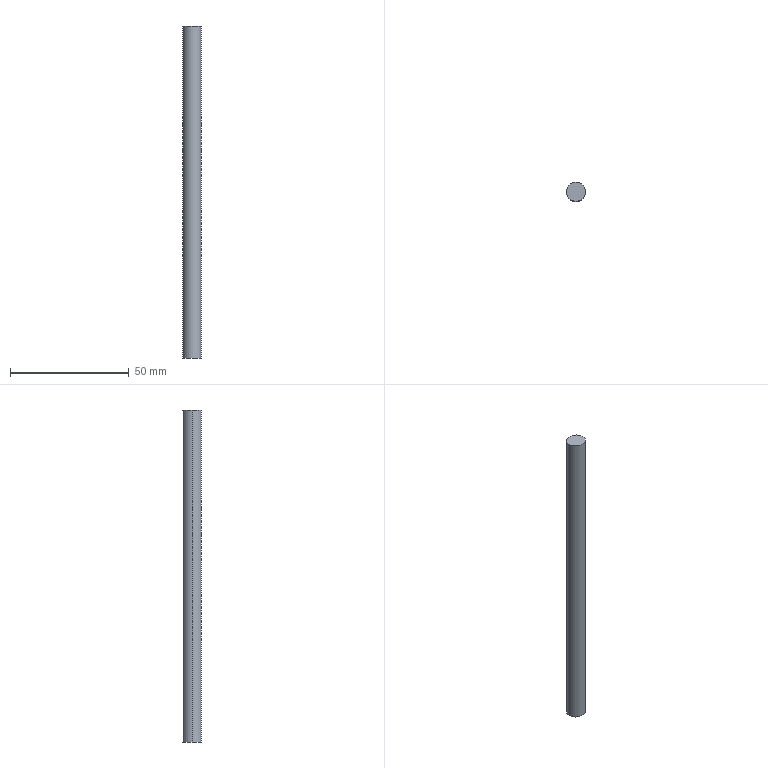Part | SolidWorks | features Extrusion 1 | 1 solid | 4 faces | box 8 x 8 x 140 mm | volume 7037 mm3 | cylinder 2 | plane 2 | commonest cylinder face diameters 8 x2
STEP:
#1=CARTESIAN_POINT('',(4.,0.,70.));
#2=VERTEX_POINT('',#1);
#3=CARTESIAN_POINT('',(-4.,0.,70.));
#4=VERTEX_POINT('',#3);
#5=CARTESIAN_POINT('',(0.,0.,70.));
#6=DIRECTION('',(0.,0.,1.));
#7=DIRECTION('',(1.,0.,0.));
#8=AXIS2_PLACEMENT_3D('',#5,#6,#7);
#9=CIRCLE('',#8,4.);
#10=EDGE_CURVE('',#2,#4,#9,.T.);
#11=ORIENTED_EDGE('',*,*,#10,.F.);
#12=CARTESIAN_POINT('',(4.,0.,-70.));
#13=VERTEX_POINT('',#12);
#14=CARTESIAN_POINT('',(4.,0.,70.));
#15=DIRECTION('',(0.,0.,-1.));
#16=VECTOR('',#15,1000.);
#17=LINE('',#14,#16);
#18=EDGE_CURVE('',#2,#13,#17,.T.);
#19=ORIENTED_EDGE('',*,*,#18,.T.);
#20=CARTESIAN_POINT('',(-4.,0.,-70.));
#21=VERTEX_POINT('',#20);
#22=CARTESIAN_POINT('',(0.,0.,-70.));
#23=DIRECTION('',(0.,0.,1.));
#24=DIRECTION('',(1.,0.,0.));
#25=AXIS2_PLACEMENT_3D('',#22,#23,#24);
#26=CIRCLE('',#25,4.);
#27=EDGE_CURVE('',#13,#21,#26,.T.);
#28=ORIENTED_EDGE('',*,*,#27,.T.);
#29=CARTESIAN_POINT('',(-4.,0.,70.));
#30=DIRECTION('',(0.,0.,-1.));
#31=VECTOR('',#30,1000.);
#32=LINE('',#29,#31);
#33=EDGE_CURVE('',#4,#21,#32,.T.);
#34=ORIENTED_EDGE('',*,*,#33,.F.);
#35=EDGE_LOOP('',(#11,#19,#28,#34));
#36=FACE_OUTER_BOUND('',#35,.T.);
#37=CARTESIAN_POINT('',(0.,0.,70.));
#38=DIRECTION('',(0.,0.,-1.));
#39=DIRECTION('',(-1.,0.,0.));
#40=AXIS2_PLACEMENT_3D('',#37,#38,#39);
#41=CYLINDRICAL_SURFACE('',#40,4.);
#42=ADVANCED_FACE('',(#36),#41,.T.);
#43=ORIENTED_EDGE('',*,*,#18,.F.);
#44=CARTESIAN_POINT('',(0.,0.,70.));
#45=DIRECTION('',(0.,0.,1.));
#46=DIRECTION('',(1.,0.,0.));
#47=AXIS2_PLACEMENT_3D('',#44,#45,#46);
#48=CIRCLE('',#47,4.);
#49=EDGE_CURVE('',#4,#2,#48,.T.);
#50=ORIENTED_EDGE('',*,*,#49,.F.);
#51=ORIENTED_EDGE('',*,*,#33,.T.);
#52=CARTESIAN_POINT('',(0.,0.,-70.));
#53=DIRECTION('',(0.,0.,1.));
#54=DIRECTION('',(1.,0.,0.));
#55=AXIS2_PLACEMENT_3D('',#52,#53,#54);
#56=CIRCLE('',#55,4.);
#57=EDGE_CURVE('',#21,#13,#56,.T.);
#58=ORIENTED_EDGE('',*,*,#57,.T.);
#59=EDGE_LOOP('',(#43,#50,#51,#58));
#60=FACE_OUTER_BOUND('',#59,.T.);
#61=CARTESIAN_POINT('',(0.,0.,70.));
#62=DIRECTION('',(0.,0.,-1.));
#63=DIRECTION('',(-1.,0.,0.));
#64=AXIS2_PLACEMENT_3D('',#61,#62,#63);
#65=CYLINDRICAL_SURFACE('',#64,4.);
#66=ADVANCED_FACE('',(#60),#65,.T.);
#67=ORIENTED_EDGE('',*,*,#49,.T.);
#68=ORIENTED_EDGE('',*,*,#10,.T.);
#69=EDGE_LOOP('',(#67,#68));
#70=FACE_OUTER_BOUND('',#69,.T.);
#71=CARTESIAN_POINT('',(0.,0.,70.));
#72=DIRECTION('',(0.,0.,1.));
#73=DIRECTION('',(1.,0.,0.));
#74=AXIS2_PLACEMENT_3D('',#71,#72,#73);
#75=PLANE('',#74);
#76=ADVANCED_FACE('',(#70),#75,.T.);
#77=ORIENTED_EDGE('',*,*,#57,.F.);
#78=ORIENTED_EDGE('',*,*,#27,.F.);
#79=EDGE_LOOP('',(#77,#78));
#80=FACE_OUTER_BOUND('',#79,.T.);
#81=CARTESIAN_POINT('',(0.,0.,-70.));
#82=DIRECTION('',(0.,0.,1.));
#83=DIRECTION('',(1.,0.,0.));
#84=AXIS2_PLACEMENT_3D('',#81,#82,#83);
#85=PLANE('',#84);
#86=ADVANCED_FACE('',(#80),#85,.F.);
#87=CLOSED_SHELL('',(#42,#66,#76,#86));
#88=MANIFOLD_SOLID_BREP('',#87);
#89=CARTESIAN_POINT('',(0.,0.,0.));
#90=DIRECTION('',(0.,0.,1.));
#91=DIRECTION('',(1.,0.,0.));
#92=AXIS2_PLACEMENT_3D('',#89,#90,#91);
#93=(LENGTH_UNIT()NAMED_UNIT(*)SI_UNIT(.MILLI.,.METRE.));
#94=UNCERTAINTY_MEASURE_WITH_UNIT(LENGTH_MEASURE(0.00001),#93,'','');
#95=(NAMED_UNIT(*)PLANE_ANGLE_UNIT()SI_UNIT($,.RADIAN.));
#96=(NAMED_UNIT(*)SI_UNIT($,.STERADIAN.)SOLID_ANGLE_UNIT());
#97=(GEOMETRIC_REPRESENTATION_CONTEXT(3)GLOBAL_UNCERTAINTY_ASSIGNED_CONTEXT((#94))GLOBAL_UNIT_ASSIGNED_CONTEXT((#93,#95,#96))REPRESENTATION_CONTEXT('',''));
#98=ADVANCED_BREP_SHAPE_REPRESENTATION('',(#88,#92),#97);